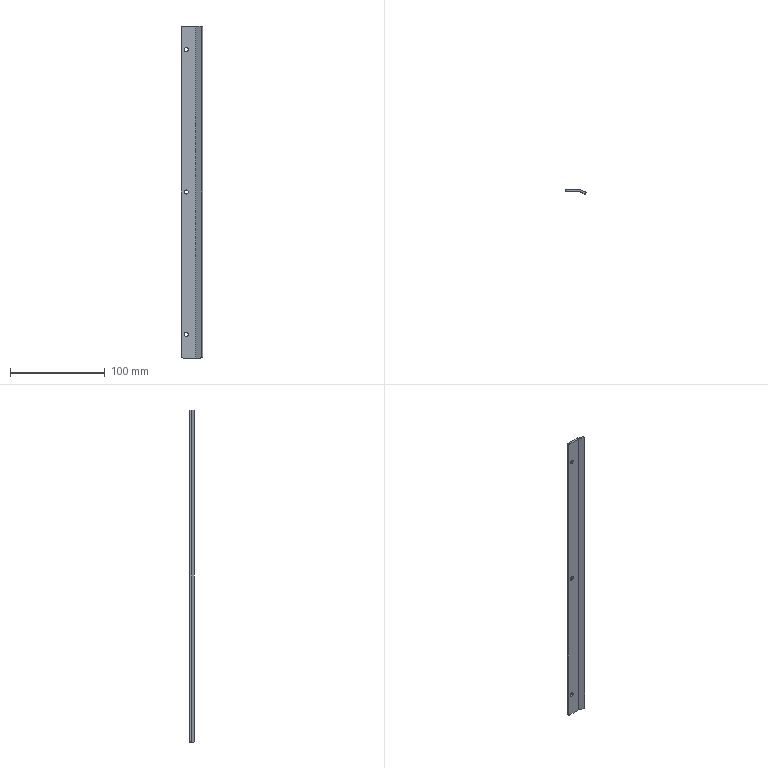Part | STEP file | 1 solid | 24 faces | box 22.338 x 5 x 350 mm | volume 15718 mm3 | cylinder 12 | plane 12 | commonest cylinder face diameters 4.3 x6 4 x4 1 x1 5 x1